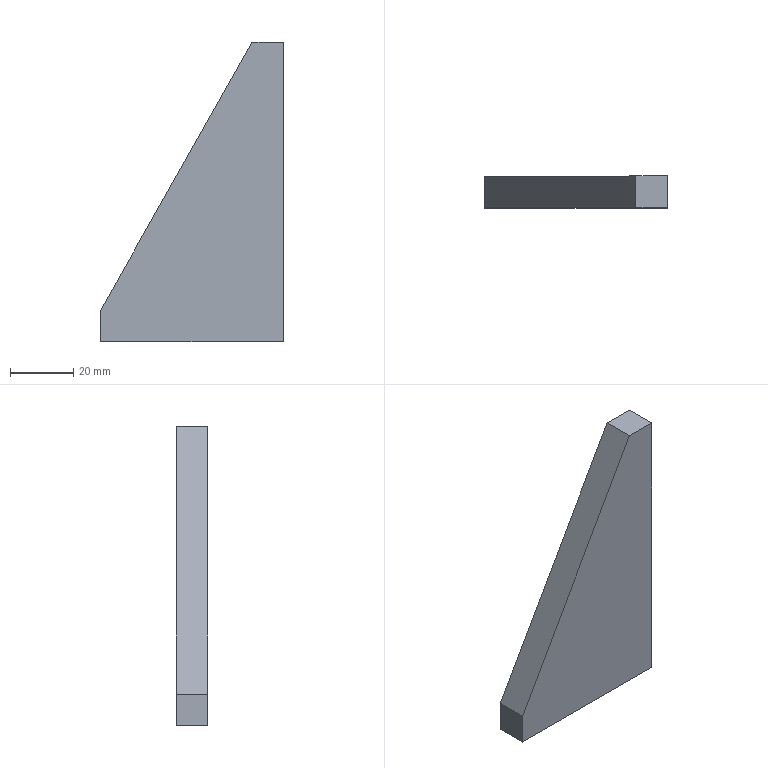Part | SolidWorks | features HoleWzd 2, Extrusion 1, ICE 1 | 1 solid | 23 faces | box 58 x 10 x 95 mm | volume 33990 mm3 | cylinder 8 | cone 8 | plane 7 | commonest cylinder face diameters 4.2 x8
STEP:
#1=CARTESIAN_POINT('',(-16.9,0.,-35.1));
#2=VERTEX_POINT('',#1);
#3=CARTESIAN_POINT('',(-21.1,0.,-35.1));
#4=VERTEX_POINT('',#3);
#5=CARTESIAN_POINT('',(-19.,0.,-35.1));
#6=DIRECTION('',(0.,0.,-1.));
#7=DIRECTION('',(-1.,0.,0.));
#8=AXIS2_PLACEMENT_3D('',#5,#6,#7);
#9=CIRCLE('',#8,2.1);
#10=EDGE_CURVE('',#2,#4,#9,.T.);
#11=ORIENTED_EDGE('',*,*,#10,.F.);
#12=CARTESIAN_POINT('',(-16.9,0.,-47.5));
#13=VERTEX_POINT('',#12);
#14=CARTESIAN_POINT('',(-16.9,0.,-47.5));
#15=DIRECTION('',(0.,0.,-1.));
#16=VECTOR('',#15,1000.);
#17=LINE('',#14,#16);
#18=EDGE_CURVE('',#2,#13,#17,.T.);
#19=ORIENTED_EDGE('',*,*,#18,.T.);
#20=CARTESIAN_POINT('',(-21.1,0.,-47.5));
#21=VERTEX_POINT('',#20);
#22=CARTESIAN_POINT('',(-19.,0.,-47.5));
#23=DIRECTION('',(0.,0.,-1.));
#24=DIRECTION('',(-1.,0.,0.));
#25=AXIS2_PLACEMENT_3D('',#22,#23,#24);
#26=CIRCLE('',#25,2.1);
#27=EDGE_CURVE('',#13,#21,#26,.T.);
#28=ORIENTED_EDGE('',*,*,#27,.T.);
#29=CARTESIAN_POINT('',(-21.1,0.,-47.5));
#30=DIRECTION('',(0.,0.,-1.));
#31=VECTOR('',#30,1000.);
#32=LINE('',#29,#31);
#33=EDGE_CURVE('',#4,#21,#32,.T.);
#34=ORIENTED_EDGE('',*,*,#33,.F.);
#35=EDGE_LOOP('',(#11,#19,#28,#34));
#36=FACE_OUTER_BOUND('',#35,.T.);
#37=CARTESIAN_POINT('',(-19.,0.,-47.5));
#38=DIRECTION('',(0.,0.,-1.));
#39=DIRECTION('',(-1.,0.,0.));
#40=AXIS2_PLACEMENT_3D('',#37,#38,#39);
#41=CYLINDRICAL_SURFACE('',#40,2.1);
#42=ADVANCED_FACE('',(#36),#41,.F.);
#43=CARTESIAN_POINT('',(-19.,0.,-33.838));
#44=VERTEX_POINT('',#43);
#45=CARTESIAN_POINT('',(-21.1,0.,-35.1));
#46=DIRECTION('',(-0.8572,0.,-0.515));
#47=VECTOR('',#46,1000.);
#48=LINE('',#45,#47);
#49=EDGE_CURVE('',#44,#4,#48,.T.);
#50=ORIENTED_EDGE('',*,*,#49,.F.);
#51=CARTESIAN_POINT('',(-16.9,0.,-35.1));
#52=DIRECTION('',(0.8572,0.,-0.515));
#53=VECTOR('',#52,1000.);
#54=LINE('',#51,#53);
#55=EDGE_CURVE('',#44,#2,#54,.T.);
#56=ORIENTED_EDGE('',*,*,#55,.T.);
#57=ORIENTED_EDGE('',*,*,#10,.T.);
#58=EDGE_LOOP('',(#50,#56,#57));
#59=FACE_OUTER_BOUND('',#58,.T.);
#60=CARTESIAN_POINT('',(-19.,0.,-35.1));
#61=DIRECTION('',(0.,0.,-1.));
#62=DIRECTION('',(-1.,0.,0.));
#63=AXIS2_PLACEMENT_3D('',#60,#61,#62);
#64=CONICAL_SURFACE('',#63,2.1,1.03);
#65=ADVANCED_FACE('',(#59),#64,.F.);
#66=CARTESIAN_POINT('',(23.1,0.,-35.1));
#67=VERTEX_POINT('',#66);
#68=CARTESIAN_POINT('',(18.9,0.,-35.1));
#69=VERTEX_POINT('',#68);
#70=CARTESIAN_POINT('',(21.,0.,-35.1));
#71=DIRECTION('',(0.,0.,-1.));
#72=DIRECTION('',(-1.,0.,0.));
#73=AXIS2_PLACEMENT_3D('',#70,#71,#72);
#74=CIRCLE('',#73,2.1);
#75=EDGE_CURVE('',#67,#69,#74,.T.);
#76=ORIENTED_EDGE('',*,*,#75,.F.);
#77=CARTESIAN_POINT('',(23.1,0.,-47.5));
#78=VERTEX_POINT('',#77);
#79=CARTESIAN_POINT('',(23.1,0.,-47.5));
#80=DIRECTION('',(0.,0.,-1.));
#81=VECTOR('',#80,1000.);
#82=LINE('',#79,#81);
#83=EDGE_CURVE('',#67,#78,#82,.T.);
#84=ORIENTED_EDGE('',*,*,#83,.T.);
#85=CARTESIAN_POINT('',(18.9,0.,-47.5));
#86=VERTEX_POINT('',#85);
#87=CARTESIAN_POINT('',(21.,0.,-47.5));
#88=DIRECTION('',(0.,0.,-1.));
#89=DIRECTION('',(-1.,0.,0.));
#90=AXIS2_PLACEMENT_3D('',#87,#88,#89);
#91=CIRCLE('',#90,2.1);
#92=EDGE_CURVE('',#78,#86,#91,.T.);
#93=ORIENTED_EDGE('',*,*,#92,.T.);
#94=CARTESIAN_POINT('',(18.9,0.,-47.5));
#95=DIRECTION('',(0.,0.,-1.));
#96=VECTOR('',#95,1000.);
#97=LINE('',#94,#96);
#98=EDGE_CURVE('',#69,#86,#97,.T.);
#99=ORIENTED_EDGE('',*,*,#98,.F.);
#100=EDGE_LOOP('',(#76,#84,#93,#99));
#101=FACE_OUTER_BOUND('',#100,.T.);
#102=CARTESIAN_POINT('',(21.,0.,-47.5));
#103=DIRECTION('',(0.,0.,-1.));
#104=DIRECTION('',(-1.,0.,0.));
#105=AXIS2_PLACEMENT_3D('',#102,#103,#104);
#106=CYLINDRICAL_SURFACE('',#105,2.1);
#107=ADVANCED_FACE('',(#101),#106,.F.);
#108=CARTESIAN_POINT('',(21.,0.,-33.838));
#109=VERTEX_POINT('',#108);
#110=CARTESIAN_POINT('',(18.9,0.,-35.1));
#111=DIRECTION('',(-0.8572,0.,-0.515));
#112=VECTOR('',#111,1000.);
#113=LINE('',#110,#112);
#114=EDGE_CURVE('',#109,#69,#113,.T.);
#115=ORIENTED_EDGE('',*,*,#114,.F.);
#116=CARTESIAN_POINT('',(23.1,0.,-35.1));
#117=DIRECTION('',(0.8572,0.,-0.515));
#118=VECTOR('',#117,1000.);
#119=LINE('',#116,#118);
#120=EDGE_CURVE('',#109,#67,#119,.T.);
#121=ORIENTED_EDGE('',*,*,#120,.T.);
#122=ORIENTED_EDGE('',*,*,#75,.T.);
#123=EDGE_LOOP('',(#115,#121,#122));
#124=FACE_OUTER_BOUND('',#123,.T.);
#125=CARTESIAN_POINT('',(21.,0.,-35.1));
#126=DIRECTION('',(0.,0.,-1.));
#127=DIRECTION('',(-1.,0.,0.));
#128=AXIS2_PLACEMENT_3D('',#125,#126,#127);
#129=CONICAL_SURFACE('',#128,2.1,1.03);
#130=ADVANCED_FACE('',(#124),#129,.F.);
#131=CARTESIAN_POINT('',(16.6,0.,39.6));
#132=VERTEX_POINT('',#131);
#133=CARTESIAN_POINT('',(16.6,0.,35.4));
#134=VERTEX_POINT('',#133);
#135=CARTESIAN_POINT('',(16.6,0.,37.5));
#136=DIRECTION('',(1.,0.,0.));
#137=DIRECTION('',(0.,0.,-1.));
#138=AXIS2_PLACEMENT_3D('',#135,#136,#137);
#139=CIRCLE('',#138,2.1);
#140=EDGE_CURVE('',#132,#134,#139,.T.);
#141=ORIENTED_EDGE('',*,*,#140,.F.);
#142=CARTESIAN_POINT('',(29.,0.,39.6));
#143=VERTEX_POINT('',#142);
#144=CARTESIAN_POINT('',(29.,0.,39.6));
#145=DIRECTION('',(1.,0.,0.));
#146=VECTOR('',#145,1000.);
#147=LINE('',#144,#146);
#148=EDGE_CURVE('',#132,#143,#147,.T.);
#149=ORIENTED_EDGE('',*,*,#148,.T.);
#150=CARTESIAN_POINT('',(29.,0.,35.4));
#151=VERTEX_POINT('',#150);
#152=CARTESIAN_POINT('',(29.,0.,37.5));
#153=DIRECTION('',(1.,0.,0.));
#154=DIRECTION('',(0.,0.,-1.));
#155=AXIS2_PLACEMENT_3D('',#152,#153,#154);
#156=CIRCLE('',#155,2.1);
#157=EDGE_CURVE('',#143,#151,#156,.T.);
#158=ORIENTED_EDGE('',*,*,#157,.T.);
#159=CARTESIAN_POINT('',(29.,0.,35.4));
#160=DIRECTION('',(1.,0.,0.));
#161=VECTOR('',#160,1000.);
#162=LINE('',#159,#161);
#163=EDGE_CURVE('',#134,#151,#162,.T.);
#164=ORIENTED_EDGE('',*,*,#163,.F.);
#165=EDGE_LOOP('',(#141,#149,#158,#164));
#166=FACE_OUTER_BOUND('',#165,.T.);
#167=CARTESIAN_POINT('',(29.,0.,37.5));
#168=DIRECTION('',(1.,0.,0.));
#169=DIRECTION('',(0.,0.,-1.));
#170=AXIS2_PLACEMENT_3D('',#167,#168,#169);
#171=CYLINDRICAL_SURFACE('',#170,2.1);
#172=ADVANCED_FACE('',(#166),#171,.F.);
#173=CARTESIAN_POINT('',(15.338,0.,37.5));
#174=VERTEX_POINT('',#173);
#175=CARTESIAN_POINT('',(16.6,0.,35.4));
#176=DIRECTION('',(0.515,0.,-0.8572));
#177=VECTOR('',#176,1000.);
#178=LINE('',#175,#177);
#179=EDGE_CURVE('',#174,#134,#178,.T.);
#180=ORIENTED_EDGE('',*,*,#179,.F.);
#181=CARTESIAN_POINT('',(16.6,0.,39.6));
#182=DIRECTION('',(0.515,0.,0.8572));
#183=VECTOR('',#182,1000.);
#184=LINE('',#181,#183);
#185=EDGE_CURVE('',#174,#132,#184,.T.);
#186=ORIENTED_EDGE('',*,*,#185,.T.);
#187=ORIENTED_EDGE('',*,*,#140,.T.);
#188=EDGE_LOOP('',(#180,#186,#187));
#189=FACE_OUTER_BOUND('',#188,.T.);
#190=CARTESIAN_POINT('',(16.6,0.,37.5));
#191=DIRECTION('',(1.,0.,0.));
#192=DIRECTION('',(0.,0.,-1.));
#193=AXIS2_PLACEMENT_3D('',#190,#191,#192);
#194=CONICAL_SURFACE('',#193,2.1,1.03);
#195=ADVANCED_FACE('',(#189),#194,.F.);
#196=CARTESIAN_POINT('',(16.6,0.,-20.4));
#197=VERTEX_POINT('',#196);
#198=CARTESIAN_POINT('',(16.6,0.,-24.6));
#199=VERTEX_POINT('',#198);
#200=CARTESIAN_POINT('',(16.6,0.,-22.5));
#201=DIRECTION('',(1.,0.,0.));
#202=DIRECTION('',(0.,0.,-1.));
#203=AXIS2_PLACEMENT_3D('',#200,#201,#202);
#204=CIRCLE('',#203,2.1);
#205=EDGE_CURVE('',#197,#199,#204,.T.);
#206=ORIENTED_EDGE('',*,*,#205,.F.);
#207=CARTESIAN_POINT('',(29.,0.,-20.4));
#208=VERTEX_POINT('',#207);
#209=CARTESIAN_POINT('',(29.,0.,-20.4));
#210=DIRECTION('',(1.,0.,0.));
#211=VECTOR('',#210,1000.);
#212=LINE('',#209,#211);
#213=EDGE_CURVE('',#197,#208,#212,.T.);
#214=ORIENTED_EDGE('',*,*,#213,.T.);
#215=CARTESIAN_POINT('',(29.,0.,-24.6));
#216=VERTEX_POINT('',#215);
#217=CARTESIAN_POINT('',(29.,0.,-22.5));
#218=DIRECTION('',(1.,0.,0.));
#219=DIRECTION('',(0.,0.,-1.));
#220=AXIS2_PLACEMENT_3D('',#217,#218,#219);
#221=CIRCLE('',#220,2.1);
#222=EDGE_CURVE('',#208,#216,#221,.T.);
#223=ORIENTED_EDGE('',*,*,#222,.T.);
#224=CARTESIAN_POINT('',(29.,0.,-24.6));
#225=DIRECTION('',(1.,0.,0.));
#226=VECTOR('',#225,1000.);
#227=LINE('',#224,#226);
#228=EDGE_CURVE('',#199,#216,#227,.T.);
#229=ORIENTED_EDGE('',*,*,#228,.F.);
#230=EDGE_LOOP('',(#206,#214,#223,#229));
#231=FACE_OUTER_BOUND('',#230,.T.);
#232=CARTESIAN_POINT('',(29.,0.,-22.5));
#233=DIRECTION('',(1.,0.,0.));
#234=DIRECTION('',(0.,0.,-1.));
#235=AXIS2_PLACEMENT_3D('',#232,#233,#234);
#236=CYLINDRICAL_SURFACE('',#235,2.1);
#237=ADVANCED_FACE('',(#231),#236,.F.);
#238=CARTESIAN_POINT('',(15.338,0.,-22.5));
#239=VERTEX_POINT('',#238);
#240=CARTESIAN_POINT('',(16.6,0.,-24.6));
#241=DIRECTION('',(0.515,0.,-0.8572));
#242=VECTOR('',#241,1000.);
#243=LINE('',#240,#242);
#244=EDGE_CURVE('',#239,#199,#243,.T.);
#245=ORIENTED_EDGE('',*,*,#244,.F.);
#246=CARTESIAN_POINT('',(16.6,0.,-20.4));
#247=DIRECTION('',(0.515,0.,0.8572));
#248=VECTOR('',#247,1000.);
#249=LINE('',#246,#248);
#250=EDGE_CURVE('',#239,#197,#249,.T.);
#251=ORIENTED_EDGE('',*,*,#250,.T.);
#252=ORIENTED_EDGE('',*,*,#205,.T.);
#253=EDGE_LOOP('',(#245,#251,#252));
#254=FACE_OUTER_BOUND('',#253,.T.);
#255=CARTESIAN_POINT('',(16.6,0.,-22.5));
#256=DIRECTION('',(1.,0.,0.));
#257=DIRECTION('',(0.,0.,-1.));
#258=AXIS2_PLACEMENT_3D('',#255,#256,#257);
#259=CONICAL_SURFACE('',#258,2.1,1.03);
#260=ADVANCED_FACE('',(#254),#259,.F.);
#261=CARTESIAN_POINT('',(29.,0.,37.5));
#262=DIRECTION('',(1.,0.,0.));
#263=DIRECTION('',(0.,0.,-1.));
#264=AXIS2_PLACEMENT_3D('',#261,#262,#263);
#265=CIRCLE('',#264,2.1);
#266=EDGE_CURVE('',#151,#143,#265,.T.);
#267=ORIENTED_EDGE('',*,*,#266,.F.);
#268=ORIENTED_EDGE('',*,*,#157,.F.);
#269=EDGE_LOOP('',(#267,#268));
#270=FACE_BOUND('',#269,.T.);
#271=CARTESIAN_POINT('',(29.,0.,-22.5));
#272=DIRECTION('',(1.,0.,0.));
#273=DIRECTION('',(0.,0.,-1.));
#274=AXIS2_PLACEMENT_3D('',#271,#272,#273);
#275=CIRCLE('',#274,2.1);
#276=EDGE_CURVE('',#216,#208,#275,.T.);
#277=ORIENTED_EDGE('',*,*,#276,.F.);
#278=ORIENTED_EDGE('',*,*,#222,.F.);
#279=EDGE_LOOP('',(#277,#278));
#280=FACE_BOUND('',#279,.T.);
#281=CARTESIAN_POINT('',(29.,-5.,47.5));
#282=VERTEX_POINT('',#281);
#283=CARTESIAN_POINT('',(29.,-5.,-47.5));
#284=VERTEX_POINT('',#283);
#285=CARTESIAN_POINT('',(29.,-5.,47.5));
#286=DIRECTION('',(0.,0.,-1.));
#287=VECTOR('',#286,1000.);
#288=LINE('',#285,#287);
#289=EDGE_CURVE('',#282,#284,#288,.T.);
#290=ORIENTED_EDGE('',*,*,#289,.T.);
#291=CARTESIAN_POINT('',(29.,5.,-47.5));
#292=VERTEX_POINT('',#291);
#293=CARTESIAN_POINT('',(29.,5.,-47.5));
#294=DIRECTION('',(0.,-1.,0.));
#295=VECTOR('',#294,1000.);
#296=LINE('',#293,#295);
#297=EDGE_CURVE('',#292,#284,#296,.T.);
#298=ORIENTED_EDGE('',*,*,#297,.F.);
#299=CARTESIAN_POINT('',(29.,5.,47.5));
#300=VERTEX_POINT('',#299);
#301=CARTESIAN_POINT('',(29.,5.,47.5));
#302=DIRECTION('',(0.,0.,-1.));
#303=VECTOR('',#302,1000.);
#304=LINE('',#301,#303);
#305=EDGE_CURVE('',#300,#292,#304,.T.);
#306=ORIENTED_EDGE('',*,*,#305,.F.);
#307=CARTESIAN_POINT('',(29.,5.,47.5));
#308=DIRECTION('',(0.,-1.,0.));
#309=VECTOR('',#308,1000.);
#310=LINE('',#307,#309);
#311=EDGE_CURVE('',#300,#282,#310,.T.);
#312=ORIENTED_EDGE('',*,*,#311,.T.);
#313=EDGE_LOOP('',(#290,#298,#306,#312));
#314=FACE_OUTER_BOUND('',#313,.T.);
#315=CARTESIAN_POINT('',(29.,5.,47.5));
#316=DIRECTION('',(-1.,0.,0.));
#317=DIRECTION('',(0.,0.,1.));
#318=AXIS2_PLACEMENT_3D('',#315,#316,#317);
#319=PLANE('',#318);
#320=ADVANCED_FACE('',(#270,#280,#314),#319,.F.);
#321=CARTESIAN_POINT('',(-19.,0.,-47.5));
#322=DIRECTION('',(0.,0.,-1.));
#323=DIRECTION('',(-1.,0.,0.));
#324=AXIS2_PLACEMENT_3D('',#321,#322,#323);
#325=CIRCLE('',#324,2.1);
#326=EDGE_CURVE('',#21,#13,#325,.T.);
#327=ORIENTED_EDGE('',*,*,#326,.F.);
#328=ORIENTED_EDGE('',*,*,#27,.F.);
#329=EDGE_LOOP('',(#327,#328));
#330=FACE_BOUND('',#329,.T.);
#331=CARTESIAN_POINT('',(21.,0.,-47.5));
#332=DIRECTION('',(0.,0.,-1.));
#333=DIRECTION('',(-1.,0.,0.));
#334=AXIS2_PLACEMENT_3D('',#331,#332,#333);
#335=CIRCLE('',#334,2.1);
#336=EDGE_CURVE('',#86,#78,#335,.T.);
#337=ORIENTED_EDGE('',*,*,#336,.F.);
#338=ORIENTED_EDGE('',*,*,#92,.F.);
#339=EDGE_LOOP('',(#337,#338));
#340=FACE_BOUND('',#339,.T.);
#341=CARTESIAN_POINT('',(-29.,-5.,-47.5));
#342=VERTEX_POINT('',#341);
#343=CARTESIAN_POINT('',(-29.,-5.,-47.5));
#344=DIRECTION('',(-1.,0.,0.));
#345=VECTOR('',#344,1000.);
#346=LINE('',#343,#345);
#347=EDGE_CURVE('',#284,#342,#346,.T.);
#348=ORIENTED_EDGE('',*,*,#347,.T.);
#349=CARTESIAN_POINT('',(-29.,5.,-47.5));
#350=VERTEX_POINT('',#349);
#351=CARTESIAN_POINT('',(-29.,5.,-47.5));
#352=DIRECTION('',(0.,-1.,0.));
#353=VECTOR('',#352,1000.);
#354=LINE('',#351,#353);
#355=EDGE_CURVE('',#350,#342,#354,.T.);
#356=ORIENTED_EDGE('',*,*,#355,.F.);
#357=CARTESIAN_POINT('',(-29.,5.,-47.5));
#358=DIRECTION('',(-1.,0.,0.));
#359=VECTOR('',#358,1000.);
#360=LINE('',#357,#359);
#361=EDGE_CURVE('',#292,#350,#360,.T.);
#362=ORIENTED_EDGE('',*,*,#361,.F.);
#363=ORIENTED_EDGE('',*,*,#297,.T.);
#364=EDGE_LOOP('',(#348,#356,#362,#363));
#365=FACE_OUTER_BOUND('',#364,.T.);
#366=CARTESIAN_POINT('',(-29.,5.,-47.5));
#367=DIRECTION('',(0.,0.,1.));
#368=DIRECTION('',(1.,0.,0.));
#369=AXIS2_PLACEMENT_3D('',#366,#367,#368);
#370=PLANE('',#369);
#371=ADVANCED_FACE('',(#330,#340,#365),#370,.F.);
#372=CARTESIAN_POINT('',(-29.,-5.,-37.5));
#373=VERTEX_POINT('',#372);
#374=CARTESIAN_POINT('',(-29.,-5.,47.5));
#375=DIRECTION('',(0.,0.,1.));
#376=VECTOR('',#375,1000.);
#377=LINE('',#374,#376);
#378=EDGE_CURVE('',#342,#373,#377,.T.);
#379=ORIENTED_EDGE('',*,*,#378,.T.);
#380=CARTESIAN_POINT('',(-29.,5.,-37.5));
#381=VERTEX_POINT('',#380);
#382=CARTESIAN_POINT('',(-29.,-102.617,-37.5));
#383=DIRECTION('',(0.,1.,0.));
#384=VECTOR('',#383,1000.);
#385=LINE('',#382,#384);
#386=EDGE_CURVE('',#373,#381,#385,.T.);
#387=ORIENTED_EDGE('',*,*,#386,.T.);
#388=CARTESIAN_POINT('',(-29.,5.,47.5));
#389=DIRECTION('',(0.,0.,1.));
#390=VECTOR('',#389,1000.);
#391=LINE('',#388,#390);
#392=EDGE_CURVE('',#350,#381,#391,.T.);
#393=ORIENTED_EDGE('',*,*,#392,.F.);
#394=ORIENTED_EDGE('',*,*,#355,.T.);
#395=EDGE_LOOP('',(#379,#387,#393,#394));
#396=FACE_OUTER_BOUND('',#395,.T.);
#397=CARTESIAN_POINT('',(-29.,5.,47.5));
#398=DIRECTION('',(1.,0.,0.));
#399=DIRECTION('',(0.,0.,-1.));
#400=AXIS2_PLACEMENT_3D('',#397,#398,#399);
#401=PLANE('',#400);
#402=ADVANCED_FACE('',(#396),#401,.F.);
#403=CARTESIAN_POINT('',(19.,5.,47.5));
#404=VERTEX_POINT('',#403);
#405=CARTESIAN_POINT('',(-29.,5.,47.5));
#406=DIRECTION('',(1.,0.,0.));
#407=VECTOR('',#406,1000.);
#408=LINE('',#405,#407);
#409=EDGE_CURVE('',#404,#300,#408,.T.);
#410=ORIENTED_EDGE('',*,*,#409,.F.);
#411=CARTESIAN_POINT('',(19.,-5.,47.5));
#412=VERTEX_POINT('',#411);
#413=CARTESIAN_POINT('',(19.,-102.617,47.5));
#414=DIRECTION('',(0.,1.,0.));
#415=VECTOR('',#414,1000.);
#416=LINE('',#413,#415);
#417=EDGE_CURVE('',#412,#404,#416,.T.);
#418=ORIENTED_EDGE('',*,*,#417,.F.);
#419=CARTESIAN_POINT('',(-29.,-5.,47.5));
#420=DIRECTION('',(1.,0.,0.));
#421=VECTOR('',#420,1000.);
#422=LINE('',#419,#421);
#423=EDGE_CURVE('',#412,#282,#422,.T.);
#424=ORIENTED_EDGE('',*,*,#423,.T.);
#425=ORIENTED_EDGE('',*,*,#311,.F.);
#426=EDGE_LOOP('',(#410,#418,#424,#425));
#427=FACE_OUTER_BOUND('',#426,.T.);
#428=CARTESIAN_POINT('',(-29.,5.,47.5));
#429=DIRECTION('',(0.,0.,-1.));
#430=DIRECTION('',(-1.,0.,0.));
#431=AXIS2_PLACEMENT_3D('',#428,#429,#430);
#432=PLANE('',#431);
#433=ADVANCED_FACE('',(#427),#432,.F.);
#434=ORIENTED_EDGE('',*,*,#392,.T.);
#435=CARTESIAN_POINT('',(19.,5.,47.5));
#436=DIRECTION('',(-0.4917,0.,-0.8708));
#437=VECTOR('',#436,1000.);
#438=LINE('',#435,#437);
#439=EDGE_CURVE('',#404,#381,#438,.T.);
#440=ORIENTED_EDGE('',*,*,#439,.F.);
#441=ORIENTED_EDGE('',*,*,#409,.T.);
#442=ORIENTED_EDGE('',*,*,#305,.T.);
#443=ORIENTED_EDGE('',*,*,#361,.T.);
#444=EDGE_LOOP('',(#434,#440,#441,#442,#443));
#445=FACE_OUTER_BOUND('',#444,.T.);
#446=CARTESIAN_POINT('',(0.,5.,0.));
#447=DIRECTION('',(0.,-1.,0.));
#448=DIRECTION('',(0.,0.,-1.));
#449=AXIS2_PLACEMENT_3D('',#446,#447,#448);
#450=PLANE('',#449);
#451=ADVANCED_FACE('',(#445),#450,.F.);
#452=CARTESIAN_POINT('',(19.,-5.,47.5));
#453=DIRECTION('',(-0.4917,0.,-0.8708));
#454=VECTOR('',#453,1000.);
#455=LINE('',#452,#454);
#456=EDGE_CURVE('',#412,#373,#455,.T.);
#457=ORIENTED_EDGE('',*,*,#456,.T.);
#458=ORIENTED_EDGE('',*,*,#378,.F.);
#459=ORIENTED_EDGE('',*,*,#347,.F.);
#460=ORIENTED_EDGE('',*,*,#289,.F.);
#461=ORIENTED_EDGE('',*,*,#423,.F.);
#462=EDGE_LOOP('',(#457,#458,#459,#460,#461));
#463=FACE_OUTER_BOUND('',#462,.T.);
#464=CARTESIAN_POINT('',(0.,-5.,0.));
#465=DIRECTION('',(0.,-1.,0.));
#466=DIRECTION('',(0.,0.,-1.));
#467=AXIS2_PLACEMENT_3D('',#464,#465,#466);
#468=PLANE('',#467);
#469=ADVANCED_FACE('',(#463),#468,.T.);
#470=ORIENTED_EDGE('',*,*,#417,.T.);
#471=ORIENTED_EDGE('',*,*,#439,.T.);
#472=ORIENTED_EDGE('',*,*,#386,.F.);
#473=ORIENTED_EDGE('',*,*,#456,.F.);
#474=EDGE_LOOP('',(#470,#471,#472,#473));
#475=FACE_OUTER_BOUND('',#474,.T.);
#476=CARTESIAN_POINT('',(19.,-102.617,47.5));
#477=DIRECTION('',(0.8708,0.,-0.4917));
#478=DIRECTION('',(-0.4917,0.,-0.8708));
#479=AXIS2_PLACEMENT_3D('',#476,#477,#478);
#480=PLANE('',#479);
#481=ADVANCED_FACE('',(#475),#480,.F.);
#482=ORIENTED_EDGE('',*,*,#250,.F.);
#483=ORIENTED_EDGE('',*,*,#244,.T.);
#484=CARTESIAN_POINT('',(16.6,0.,-22.5));
#485=DIRECTION('',(1.,0.,0.));
#486=DIRECTION('',(0.,0.,-1.));
#487=AXIS2_PLACEMENT_3D('',#484,#485,#486);
#488=CIRCLE('',#487,2.1);
#489=EDGE_CURVE('',#199,#197,#488,.T.);
#490=ORIENTED_EDGE('',*,*,#489,.T.);
#491=EDGE_LOOP('',(#482,#483,#490));
#492=FACE_OUTER_BOUND('',#491,.T.);
#493=CARTESIAN_POINT('',(16.6,0.,-22.5));
#494=DIRECTION('',(1.,0.,0.));
#495=DIRECTION('',(0.,0.,-1.));
#496=AXIS2_PLACEMENT_3D('',#493,#494,#495);
#497=CONICAL_SURFACE('',#496,2.1,1.03);
#498=ADVANCED_FACE('',(#492),#497,.F.);
#499=ORIENTED_EDGE('',*,*,#213,.F.);
#500=ORIENTED_EDGE('',*,*,#489,.F.);
#501=ORIENTED_EDGE('',*,*,#228,.T.);
#502=ORIENTED_EDGE('',*,*,#276,.T.);
#503=EDGE_LOOP('',(#499,#500,#501,#502));
#504=FACE_OUTER_BOUND('',#503,.T.);
#505=CARTESIAN_POINT('',(29.,0.,-22.5));
#506=DIRECTION('',(1.,0.,0.));
#507=DIRECTION('',(0.,0.,-1.));
#508=AXIS2_PLACEMENT_3D('',#505,#506,#507);
#509=CYLINDRICAL_SURFACE('',#508,2.1);
#510=ADVANCED_FACE('',(#504),#509,.F.);
#511=ORIENTED_EDGE('',*,*,#185,.F.);
#512=ORIENTED_EDGE('',*,*,#179,.T.);
#513=CARTESIAN_POINT('',(16.6,0.,37.5));
#514=DIRECTION('',(1.,0.,0.));
#515=DIRECTION('',(0.,0.,-1.));
#516=AXIS2_PLACEMENT_3D('',#513,#514,#515);
#517=CIRCLE('',#516,2.1);
#518=EDGE_CURVE('',#134,#132,#517,.T.);
#519=ORIENTED_EDGE('',*,*,#518,.T.);
#520=EDGE_LOOP('',(#511,#512,#519));
#521=FACE_OUTER_BOUND('',#520,.T.);
#522=CARTESIAN_POINT('',(16.6,0.,37.5));
#523=DIRECTION('',(1.,0.,0.));
#524=DIRECTION('',(0.,0.,-1.));
#525=AXIS2_PLACEMENT_3D('',#522,#523,#524);
#526=CONICAL_SURFACE('',#525,2.1,1.03);
#527=ADVANCED_FACE('',(#521),#526,.F.);
#528=ORIENTED_EDGE('',*,*,#148,.F.);
#529=ORIENTED_EDGE('',*,*,#518,.F.);
#530=ORIENTED_EDGE('',*,*,#163,.T.);
#531=ORIENTED_EDGE('',*,*,#266,.T.);
#532=EDGE_LOOP('',(#528,#529,#530,#531));
#533=FACE_OUTER_BOUND('',#532,.T.);
#534=CARTESIAN_POINT('',(29.,0.,37.5));
#535=DIRECTION('',(1.,0.,0.));
#536=DIRECTION('',(0.,0.,-1.));
#537=AXIS2_PLACEMENT_3D('',#534,#535,#536);
#538=CYLINDRICAL_SURFACE('',#537,2.1);
#539=ADVANCED_FACE('',(#533),#538,.F.);
#540=ORIENTED_EDGE('',*,*,#120,.F.);
#541=ORIENTED_EDGE('',*,*,#114,.T.);
#542=CARTESIAN_POINT('',(21.,0.,-35.1));
#543=DIRECTION('',(0.,0.,-1.));
#544=DIRECTION('',(-1.,0.,0.));
#545=AXIS2_PLACEMENT_3D('',#542,#543,#544);
#546=CIRCLE('',#545,2.1);
#547=EDGE_CURVE('',#69,#67,#546,.T.);
#548=ORIENTED_EDGE('',*,*,#547,.T.);
#549=EDGE_LOOP('',(#540,#541,#548));
#550=FACE_OUTER_BOUND('',#549,.T.);
#551=CARTESIAN_POINT('',(21.,0.,-35.1));
#552=DIRECTION('',(0.,0.,-1.));
#553=DIRECTION('',(-1.,0.,0.));
#554=AXIS2_PLACEMENT_3D('',#551,#552,#553);
#555=CONICAL_SURFACE('',#554,2.1,1.03);
#556=ADVANCED_FACE('',(#550),#555,.F.);
#557=ORIENTED_EDGE('',*,*,#83,.F.);
#558=ORIENTED_EDGE('',*,*,#547,.F.);
#559=ORIENTED_EDGE('',*,*,#98,.T.);
#560=ORIENTED_EDGE('',*,*,#336,.T.);
#561=EDGE_LOOP('',(#557,#558,#559,#560));
#562=FACE_OUTER_BOUND('',#561,.T.);
#563=CARTESIAN_POINT('',(21.,0.,-47.5));
#564=DIRECTION('',(0.,0.,-1.));
#565=DIRECTION('',(-1.,0.,0.));
#566=AXIS2_PLACEMENT_3D('',#563,#564,#565);
#567=CYLINDRICAL_SURFACE('',#566,2.1);
#568=ADVANCED_FACE('',(#562),#567,.F.);
#569=ORIENTED_EDGE('',*,*,#55,.F.);
#570=ORIENTED_EDGE('',*,*,#49,.T.);
#571=CARTESIAN_POINT('',(-19.,0.,-35.1));
#572=DIRECTION('',(0.,0.,-1.));
#573=DIRECTION('',(-1.,0.,0.));
#574=AXIS2_PLACEMENT_3D('',#571,#572,#573);
#575=CIRCLE('',#574,2.1);
#576=EDGE_CURVE('',#4,#2,#575,.T.);
#577=ORIENTED_EDGE('',*,*,#576,.T.);
#578=EDGE_LOOP('',(#569,#570,#577));
#579=FACE_OUTER_BOUND('',#578,.T.);
#580=CARTESIAN_POINT('',(-19.,0.,-35.1));
#581=DIRECTION('',(0.,0.,-1.));
#582=DIRECTION('',(-1.,0.,0.));
#583=AXIS2_PLACEMENT_3D('',#580,#581,#582);
#584=CONICAL_SURFACE('',#583,2.1,1.03);
#585=ADVANCED_FACE('',(#579),#584,.F.);
#586=ORIENTED_EDGE('',*,*,#18,.F.);
#587=ORIENTED_EDGE('',*,*,#576,.F.);
#588=ORIENTED_EDGE('',*,*,#33,.T.);
#589=ORIENTED_EDGE('',*,*,#326,.T.);
#590=EDGE_LOOP('',(#586,#587,#588,#589));
#591=FACE_OUTER_BOUND('',#590,.T.);
#592=CARTESIAN_POINT('',(-19.,0.,-47.5));
#593=DIRECTION('',(0.,0.,-1.));
#594=DIRECTION('',(-1.,0.,0.));
#595=AXIS2_PLACEMENT_3D('',#592,#593,#594);
#596=CYLINDRICAL_SURFACE('',#595,2.1);
#597=ADVANCED_FACE('',(#591),#596,.F.);
#598=CLOSED_SHELL('',(#42,#65,#107,#130,#172,#195,#237,#260,#320,#371,#402,#433,#451,#469,#481,#498,#510,#527,#539,#556,#568,#585,#597));
#599=MANIFOLD_SOLID_BREP('',#598);
#600=CARTESIAN_POINT('',(0.,0.,0.));
#601=DIRECTION('',(0.,0.,1.));
#602=DIRECTION('',(1.,0.,0.));
#603=AXIS2_PLACEMENT_3D('',#600,#601,#602);
#604=(LENGTH_UNIT()NAMED_UNIT(*)SI_UNIT(.MILLI.,.METRE.));
#605=UNCERTAINTY_MEASURE_WITH_UNIT(LENGTH_MEASURE(0.00001),#604,'','');
#606=(NAMED_UNIT(*)PLANE_ANGLE_UNIT()SI_UNIT($,.RADIAN.));
#607=(NAMED_UNIT(*)SI_UNIT($,.STERADIAN.)SOLID_ANGLE_UNIT());
#608=(GEOMETRIC_REPRESENTATION_CONTEXT(3)GLOBAL_UNCERTAINTY_ASSIGNED_CONTEXT((#605))GLOBAL_UNIT_ASSIGNED_CONTEXT((#604,#606,#607))REPRESENTATION_CONTEXT('',''));
#609=ADVANCED_BREP_SHAPE_REPRESENTATION('',(#599,#603),#608);